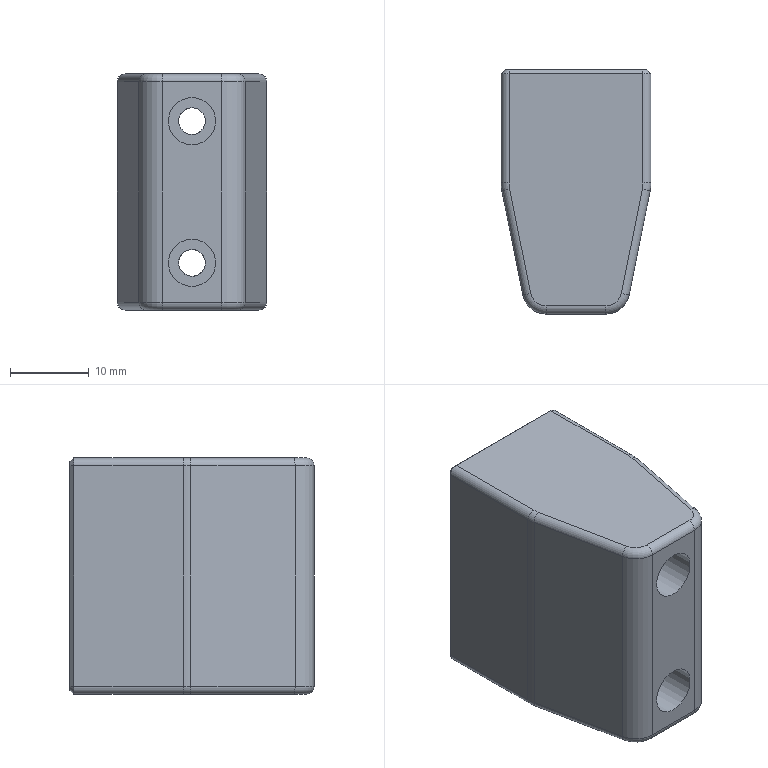CAM job | NX | 3+2 milling, drilling | part box 19 x 31 x 30 mm | stock box 20 x 36 x 35 mm
Tools:
number,name,description,diameter,corner_radius,flute_length,length,flutes
18,D2,平底铣刀-粗,2.0,0.0,50.0,75.0,2
3,D3,平底铣刀-粗,3.0,0.0,20.0,75.0,2
9,D10,平底铣刀-粗,10.0,0.0,35.0,75.0,2
19,D2-J,平底铣刀-精,2.0,0.0,50.0,75.0,2
10,D10-J,平底铣刀-精,10.0,0.0,35.0,75.0,2
19,D6R0.5,圆鼻刀-粗,6.0,0.5,50.0,75.0,2
1,D80R0.8飞刀,圆鼻刀-粗,80.0,0.8,50.0,75.0,2
1,D80R0.8飞刀-J,圆鼻刀-精,80.0,0.8,50.0,75.0,2
2,D6倒角刀,倒角刀,6.0,0.0,3.0,25.0,2
17,ZT2.8,钻头,2.8,0.0,35.0,50.0,2
13,ZT3.4,钻头,3.4,0.0,35.0,50.0,2
Operations:
program,operation,operation_type,tool,method,geometry_group,spindle_rpm,surface_speed,feed_per_tooth,feed_cut,feed_plunge,cut_length_mm,path_length_mm,cut_time_min,machine_time_min
B,底壁铣飞面一刀开粗_COPY,VolumeBased25DMillingOperation,D80R0.8飞刀,分层开粗-切深K-步距G,W-B,2800.0,703.696,0.5357,3000.0,100.0,1243.746,2515.967,0.4146,0.5418
B,底壁铣飞面一刀精光_COPY,VolumeBased25DMillingOperation,D80R0.8飞刀-J,侧刃精光-切深K-步距G,W-B,4000.0,1005.28,0.125,1000.0,100.0,137.998,173.998,0.138,0.1416
B,等高精光往复爬面_COPY,ZLevelMilling,D10,等高爬面-切深K-步距G,W-B,7000.0,219.911,0.2857,4000.0,100.0,10308.283,10403.939,2.577,2.587
B,铣沉头_1,CylinderMilling,D3,METHOD,W-B,6000.0,56.549,0.0917,1100.0,100.0,1372.595,1499.995,1.248,1.261
B,铣孔_1,CylinderMilling,D3,METHOD,W-B,6000.0,56.549,0.025,300.0,100.0,107.404,265.404,0.358,0.3738
B,铣倒角_1,PlanarMilling,D6倒角刀,METHOD,W-B,7000.0,131.947,0.0429,600.0,100.0,21.936,125.94,0.0366,0.047
B,等高精光往复爬面_COPY_COPY,ZLevelMilling,D6R0.5,等高爬面-切深K-步距G,W-B,7000.0,131.947,0.3214,4500.0,100.0,18507.703,18636.275,4.113,4.126
B,等高精光往复爬面_COPY_COPY_COPY,ZLevelMilling,D6R0.5,等高爬面-切深K-步距G,W-B,7000.0,131.947,0.3214,4500.0,100.0,459.437,556.341,0.1021,0.1118
A,顶面,FaceMilling,D80R0.8飞刀,侧刃精光-切深K-步距G,W-A,5000.0,1256.637,0.1,1000.0,100.0,124.0,160.0,0.124,0.1276
A,外形粗_2,VolumeBased25DMillingOperation,D10,METHOD,W-A,8000.0,251.327,0.3125,5000.0,80.0,5263.044,5332.844,1.053,1.06
A,打点-深0.8,Operation,D6倒角刀,NONE,W-A,8000.0,150.796,0.0312,500.0,90.0,7.2,89.988,0.0144,0.0227
A,通孔-3-4,Operation,ZT3.4,NONE,W-A,3000.0,32.044,0.0333,200.0,90.0,70.0,199.028,0.35,0.3629
A,盲锥孔-精孔3.0预钻,Operation,ZT2.8,NONE,W-A,3000.0,26.389,0.0333,200.0,90.0,19.603,92.247,0.098,0.1053
A,铣孔开粗D2_1,CylinderMilling,D2,NONE,W-A,8000.0,50.266,0.0312,500.0,100.0,103.815,210.815,0.2076,0.2183
A,钻倒角_1,Operation,D6倒角刀,METHOD,W-A,8000.0,150.796,0.0312,500.0,0.0,9.6,74.569,0.0192,0.0257
A,钻倒角_2,Operation,D6倒角刀,METHOD,W-A,8000.0,150.796,0.0312,500.0,0.0,10.0,81.248,0.02,0.0271
A,底壁铣倒角_COPY,VolumeBased25DMillingOperation,D6倒角刀,爬面_倒角-切深0-步距G,W-A,6500.0,122.519,0.1154,1500.0,100.0,107.601,147.001,0.0717,0.0757
A,铣孔精光D2_1,CylinderMilling,D2-J,精光步距切深关,W-A,8000.0,50.266,0.0125,200.0,100.0,66.341,173.341,0.3317,0.3424
A,外形半精_2,VolumeBased25DMillingOperation,D10-J,METHOD,W-A,8000.0,251.327,0.0625,1000.0,100.0,265.339,439.752,0.2653,0.2828